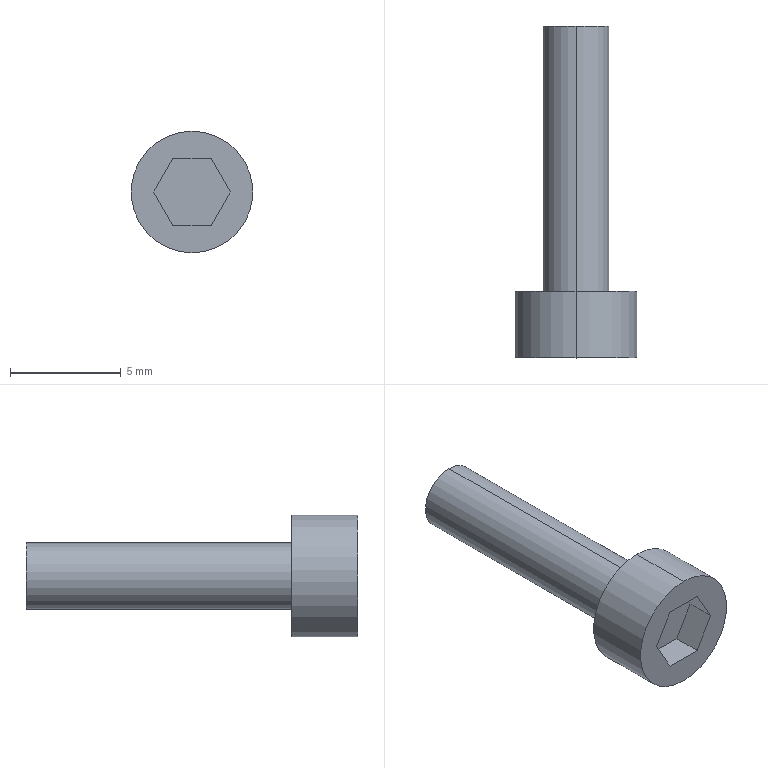Part | SolidWorks | features BaseBody 1 | 1 solid | 14 faces | box 5.5 x 15 x 5.5 mm | volume 145.965 mm3 | plane 10 | cylinder 4 | commonest cylinder face diameters 3 x2 5.5 x2
STEP:
#1=CARTESIAN_POINT('',(0.,15.,-1.5));
#2=VERTEX_POINT('',#1);
#3=CARTESIAN_POINT('',(0.,15.,1.5));
#4=VERTEX_POINT('',#3);
#5=CARTESIAN_POINT('',(0.,15.,0.));
#6=DIRECTION('',(0.,-1.,0.));
#7=DIRECTION('',(0.,0.,-1.));
#8=AXIS2_PLACEMENT_3D('',#5,#6,#7);
#9=CIRCLE('',#8,1.5);
#10=EDGE_CURVE('',#2,#4,#9,.T.);
#11=ORIENTED_EDGE('',*,*,#10,.T.);
#12=CARTESIAN_POINT('',(0.,3.,1.5));
#13=VERTEX_POINT('',#12);
#14=CARTESIAN_POINT('',(0.,15.,1.5));
#15=DIRECTION('',(0.,-1.,0.));
#16=VECTOR('',#15,1000.);
#17=LINE('',#14,#16);
#18=EDGE_CURVE('',#4,#13,#17,.T.);
#19=ORIENTED_EDGE('',*,*,#18,.T.);
#20=CARTESIAN_POINT('',(0.,3.,-1.5));
#21=VERTEX_POINT('',#20);
#22=CARTESIAN_POINT('',(0.,3.,0.));
#23=DIRECTION('',(0.,1.,0.));
#24=DIRECTION('',(0.,0.,-1.));
#25=AXIS2_PLACEMENT_3D('',#22,#23,#24);
#26=CIRCLE('',#25,1.5);
#27=EDGE_CURVE('',#13,#21,#26,.T.);
#28=ORIENTED_EDGE('',*,*,#27,.T.);
#29=CARTESIAN_POINT('',(0.,15.,-1.5));
#30=DIRECTION('',(0.,-1.,0.));
#31=VECTOR('',#30,1000.);
#32=LINE('',#29,#31);
#33=EDGE_CURVE('',#2,#21,#32,.T.);
#34=ORIENTED_EDGE('',*,*,#33,.F.);
#35=EDGE_LOOP('',(#11,#19,#28,#34));
#36=FACE_OUTER_BOUND('',#35,.T.);
#37=CARTESIAN_POINT('',(0.,15.,0.));
#38=DIRECTION('',(0.,-1.,0.));
#39=DIRECTION('',(0.,0.,-1.));
#40=AXIS2_PLACEMENT_3D('',#37,#38,#39);
#41=CYLINDRICAL_SURFACE('',#40,1.5);
#42=ADVANCED_FACE('',(#36),#41,.T.);
#43=CARTESIAN_POINT('',(0.,3.,2.75));
#44=VERTEX_POINT('',#43);
#45=CARTESIAN_POINT('',(0.,3.,-2.75));
#46=VERTEX_POINT('',#45);
#47=CARTESIAN_POINT('',(0.,3.,0.));
#48=DIRECTION('',(0.,1.,0.));
#49=DIRECTION('',(0.,0.,-1.));
#50=AXIS2_PLACEMENT_3D('',#47,#48,#49);
#51=CIRCLE('',#50,2.75);
#52=EDGE_CURVE('',#44,#46,#51,.T.);
#53=ORIENTED_EDGE('',*,*,#52,.F.);
#54=CARTESIAN_POINT('',(0.,0.,2.75));
#55=VERTEX_POINT('',#54);
#56=CARTESIAN_POINT('',(0.,3.,2.75));
#57=DIRECTION('',(0.,-1.,0.));
#58=VECTOR('',#57,1000.);
#59=LINE('',#56,#58);
#60=EDGE_CURVE('',#44,#55,#59,.T.);
#61=ORIENTED_EDGE('',*,*,#60,.T.);
#62=CARTESIAN_POINT('',(0.,0.,-2.75));
#63=VERTEX_POINT('',#62);
#64=CARTESIAN_POINT('',(0.,0.,0.));
#65=DIRECTION('',(0.,1.,0.));
#66=DIRECTION('',(0.,0.,-1.));
#67=AXIS2_PLACEMENT_3D('',#64,#65,#66);
#68=CIRCLE('',#67,2.75);
#69=EDGE_CURVE('',#55,#63,#68,.T.);
#70=ORIENTED_EDGE('',*,*,#69,.T.);
#71=CARTESIAN_POINT('',(0.,3.,-2.75));
#72=DIRECTION('',(0.,-1.,0.));
#73=VECTOR('',#72,1000.);
#74=LINE('',#71,#73);
#75=EDGE_CURVE('',#46,#63,#74,.T.);
#76=ORIENTED_EDGE('',*,*,#75,.F.);
#77=EDGE_LOOP('',(#53,#61,#70,#76));
#78=FACE_OUTER_BOUND('',#77,.T.);
#79=CARTESIAN_POINT('',(0.,3.,0.));
#80=DIRECTION('',(0.,-1.,0.));
#81=DIRECTION('',(0.,0.,-1.));
#82=AXIS2_PLACEMENT_3D('',#79,#80,#81);
#83=CYLINDRICAL_SURFACE('',#82,2.75);
#84=ADVANCED_FACE('',(#78),#83,.T.);
#85=ORIENTED_EDGE('',*,*,#18,.F.);
#86=CARTESIAN_POINT('',(0.,15.,0.));
#87=DIRECTION('',(0.,-1.,0.));
#88=DIRECTION('',(0.,0.,-1.));
#89=AXIS2_PLACEMENT_3D('',#86,#87,#88);
#90=CIRCLE('',#89,1.5);
#91=EDGE_CURVE('',#4,#2,#90,.T.);
#92=ORIENTED_EDGE('',*,*,#91,.T.);
#93=ORIENTED_EDGE('',*,*,#33,.T.);
#94=CARTESIAN_POINT('',(0.,3.,0.));
#95=DIRECTION('',(0.,1.,0.));
#96=DIRECTION('',(0.,0.,-1.));
#97=AXIS2_PLACEMENT_3D('',#94,#95,#96);
#98=CIRCLE('',#97,1.5);
#99=EDGE_CURVE('',#21,#13,#98,.T.);
#100=ORIENTED_EDGE('',*,*,#99,.T.);
#101=EDGE_LOOP('',(#85,#92,#93,#100));
#102=FACE_OUTER_BOUND('',#101,.T.);
#103=CARTESIAN_POINT('',(0.,15.,0.));
#104=DIRECTION('',(0.,-1.,0.));
#105=DIRECTION('',(0.,0.,-1.));
#106=AXIS2_PLACEMENT_3D('',#103,#104,#105);
#107=CYLINDRICAL_SURFACE('',#106,1.5);
#108=ADVANCED_FACE('',(#102),#107,.T.);
#109=CARTESIAN_POINT('',(0.,3.,0.));
#110=DIRECTION('',(0.,1.,0.));
#111=DIRECTION('',(0.,0.,-1.));
#112=AXIS2_PLACEMENT_3D('',#109,#110,#111);
#113=CIRCLE('',#112,2.75);
#114=EDGE_CURVE('',#46,#44,#113,.T.);
#115=ORIENTED_EDGE('',*,*,#114,.T.);
#116=ORIENTED_EDGE('',*,*,#52,.T.);
#117=EDGE_LOOP('',(#115,#116));
#118=FACE_OUTER_BOUND('',#117,.T.);
#119=ORIENTED_EDGE('',*,*,#99,.F.);
#120=ORIENTED_EDGE('',*,*,#27,.F.);
#121=EDGE_LOOP('',(#119,#120));
#122=FACE_BOUND('',#121,.T.);
#123=CARTESIAN_POINT('',(0.,3.,0.));
#124=DIRECTION('',(0.,1.,0.));
#125=DIRECTION('',(0.,0.,1.));
#126=AXIS2_PLACEMENT_3D('',#123,#124,#125);
#127=PLANE('',#126);
#128=ADVANCED_FACE('',(#118,#122),#127,.T.);
#129=ORIENTED_EDGE('',*,*,#10,.F.);
#130=ORIENTED_EDGE('',*,*,#91,.F.);
#131=EDGE_LOOP('',(#129,#130));
#132=FACE_OUTER_BOUND('',#131,.T.);
#133=CARTESIAN_POINT('',(0.,15.,0.));
#134=DIRECTION('',(0.,1.,0.));
#135=DIRECTION('',(0.,0.,1.));
#136=AXIS2_PLACEMENT_3D('',#133,#134,#135);
#137=PLANE('',#136);
#138=ADVANCED_FACE('',(#132),#137,.T.);
#139=ORIENTED_EDGE('',*,*,#60,.F.);
#140=ORIENTED_EDGE('',*,*,#114,.F.);
#141=ORIENTED_EDGE('',*,*,#75,.T.);
#142=CARTESIAN_POINT('',(0.,0.,0.));
#143=DIRECTION('',(0.,1.,0.));
#144=DIRECTION('',(0.,0.,-1.));
#145=AXIS2_PLACEMENT_3D('',#142,#143,#144);
#146=CIRCLE('',#145,2.75);
#147=EDGE_CURVE('',#63,#55,#146,.T.);
#148=ORIENTED_EDGE('',*,*,#147,.T.);
#149=EDGE_LOOP('',(#139,#140,#141,#148));
#150=FACE_OUTER_BOUND('',#149,.T.);
#151=CARTESIAN_POINT('',(0.,3.,0.));
#152=DIRECTION('',(0.,-1.,0.));
#153=DIRECTION('',(0.,0.,-1.));
#154=AXIS2_PLACEMENT_3D('',#151,#152,#153);
#155=CYLINDRICAL_SURFACE('',#154,2.75);
#156=ADVANCED_FACE('',(#150),#155,.T.);
#157=ORIENTED_EDGE('',*,*,#147,.F.);
#158=ORIENTED_EDGE('',*,*,#69,.F.);
#159=EDGE_LOOP('',(#157,#158));
#160=FACE_OUTER_BOUND('',#159,.T.);
#161=CARTESIAN_POINT('',(0.866,0.,-1.5));
#162=VERTEX_POINT('',#161);
#163=CARTESIAN_POINT('',(1.732,0.,0.));
#164=VERTEX_POINT('',#163);
#165=CARTESIAN_POINT('',(0.866,0.,-1.5));
#166=DIRECTION('',(0.5,0.,0.866));
#167=VECTOR('',#166,1000.);
#168=LINE('',#165,#167);
#169=EDGE_CURVE('',#162,#164,#168,.T.);
#170=ORIENTED_EDGE('',*,*,#169,.F.);
#171=CARTESIAN_POINT('',(-0.866,0.,-1.5));
#172=VERTEX_POINT('',#171);
#173=CARTESIAN_POINT('',(0.,0.,-1.5));
#174=DIRECTION('',(1.,0.,0.));
#175=VECTOR('',#174,1000.);
#176=LINE('',#173,#175);
#177=EDGE_CURVE('',#172,#162,#176,.T.);
#178=ORIENTED_EDGE('',*,*,#177,.F.);
#179=CARTESIAN_POINT('',(-1.732,0.,0.));
#180=VERTEX_POINT('',#179);
#181=CARTESIAN_POINT('',(-1.732,0.,0.));
#182=DIRECTION('',(0.5,0.,-0.866));
#183=VECTOR('',#182,1000.);
#184=LINE('',#181,#183);
#185=EDGE_CURVE('',#180,#172,#184,.T.);
#186=ORIENTED_EDGE('',*,*,#185,.F.);
#187=CARTESIAN_POINT('',(-0.866,0.,1.5));
#188=VERTEX_POINT('',#187);
#189=CARTESIAN_POINT('',(-0.866,0.,1.5));
#190=DIRECTION('',(-0.5,0.,-0.866));
#191=VECTOR('',#190,1000.);
#192=LINE('',#189,#191);
#193=EDGE_CURVE('',#188,#180,#192,.T.);
#194=ORIENTED_EDGE('',*,*,#193,.F.);
#195=CARTESIAN_POINT('',(0.866,0.,1.5));
#196=VERTEX_POINT('',#195);
#197=CARTESIAN_POINT('',(0.,0.,1.5));
#198=DIRECTION('',(-1.,0.,0.));
#199=VECTOR('',#198,1000.);
#200=LINE('',#197,#199);
#201=EDGE_CURVE('',#196,#188,#200,.T.);
#202=ORIENTED_EDGE('',*,*,#201,.F.);
#203=CARTESIAN_POINT('',(1.732,0.,0.));
#204=DIRECTION('',(-0.5,0.,0.866));
#205=VECTOR('',#204,1000.);
#206=LINE('',#203,#205);
#207=EDGE_CURVE('',#164,#196,#206,.T.);
#208=ORIENTED_EDGE('',*,*,#207,.F.);
#209=EDGE_LOOP('',(#170,#178,#186,#194,#202,#208));
#210=FACE_BOUND('',#209,.T.);
#211=CARTESIAN_POINT('',(0.,0.,0.));
#212=DIRECTION('',(0.,1.,0.));
#213=DIRECTION('',(0.,0.,1.));
#214=AXIS2_PLACEMENT_3D('',#211,#212,#213);
#215=PLANE('',#214);
#216=ADVANCED_FACE('',(#160,#210),#215,.F.);
#217=CARTESIAN_POINT('',(0.866,1.3,1.5));
#218=VERTEX_POINT('',#217);
#219=CARTESIAN_POINT('',(0.866,1.3,1.5));
#220=DIRECTION('',(0.,-1.,0.));
#221=VECTOR('',#220,1000.);
#222=LINE('',#219,#221);
#223=EDGE_CURVE('',#218,#196,#222,.T.);
#224=ORIENTED_EDGE('',*,*,#223,.F.);
#225=CARTESIAN_POINT('',(1.732,1.3,0.));
#226=VERTEX_POINT('',#225);
#227=CARTESIAN_POINT('',(1.732,1.3,0.));
#228=DIRECTION('',(-0.5,0.,0.866));
#229=VECTOR('',#228,1000.);
#230=LINE('',#227,#229);
#231=EDGE_CURVE('',#226,#218,#230,.T.);
#232=ORIENTED_EDGE('',*,*,#231,.F.);
#233=CARTESIAN_POINT('',(1.732,1.3,0.));
#234=DIRECTION('',(0.,1.,0.));
#235=VECTOR('',#234,1000.);
#236=LINE('',#233,#235);
#237=EDGE_CURVE('',#164,#226,#236,.T.);
#238=ORIENTED_EDGE('',*,*,#237,.F.);
#239=ORIENTED_EDGE('',*,*,#207,.T.);
#240=EDGE_LOOP('',(#224,#232,#238,#239));
#241=FACE_OUTER_BOUND('',#240,.T.);
#242=CARTESIAN_POINT('',(1.732,1.3,0.));
#243=DIRECTION('',(0.866,0.,0.5));
#244=DIRECTION('',(0.5,0.,-0.866));
#245=AXIS2_PLACEMENT_3D('',#242,#243,#244);
#246=PLANE('',#245);
#247=ADVANCED_FACE('',(#241),#246,.F.);
#248=ORIENTED_EDGE('',*,*,#237,.T.);
#249=CARTESIAN_POINT('',(0.866,1.3,-1.5));
#250=VERTEX_POINT('',#249);
#251=CARTESIAN_POINT('',(0.866,1.3,-1.5));
#252=DIRECTION('',(0.5,0.,0.866));
#253=VECTOR('',#252,1000.);
#254=LINE('',#251,#253);
#255=EDGE_CURVE('',#250,#226,#254,.T.);
#256=ORIENTED_EDGE('',*,*,#255,.F.);
#257=CARTESIAN_POINT('',(0.866,1.3,-1.5));
#258=DIRECTION('',(0.,1.,0.));
#259=VECTOR('',#258,1000.);
#260=LINE('',#257,#259);
#261=EDGE_CURVE('',#162,#250,#260,.T.);
#262=ORIENTED_EDGE('',*,*,#261,.F.);
#263=ORIENTED_EDGE('',*,*,#169,.T.);
#264=EDGE_LOOP('',(#248,#256,#262,#263));
#265=FACE_OUTER_BOUND('',#264,.T.);
#266=CARTESIAN_POINT('',(0.866,1.3,-1.5));
#267=DIRECTION('',(0.866,0.,-0.5));
#268=DIRECTION('',(-0.5,0.,-0.866));
#269=AXIS2_PLACEMENT_3D('',#266,#267,#268);
#270=PLANE('',#269);
#271=ADVANCED_FACE('',(#265),#270,.F.);
#272=ORIENTED_EDGE('',*,*,#261,.T.);
#273=CARTESIAN_POINT('',(-0.866,1.3,-1.5));
#274=VERTEX_POINT('',#273);
#275=CARTESIAN_POINT('',(-0.866,1.3,-1.5));
#276=DIRECTION('',(1.,0.,0.));
#277=VECTOR('',#276,1000.);
#278=LINE('',#275,#277);
#279=EDGE_CURVE('',#274,#250,#278,.T.);
#280=ORIENTED_EDGE('',*,*,#279,.F.);
#281=CARTESIAN_POINT('',(-0.866,1.3,-1.5));
#282=DIRECTION('',(0.,1.,0.));
#283=VECTOR('',#282,1000.);
#284=LINE('',#281,#283);
#285=EDGE_CURVE('',#172,#274,#284,.T.);
#286=ORIENTED_EDGE('',*,*,#285,.F.);
#287=ORIENTED_EDGE('',*,*,#177,.T.);
#288=EDGE_LOOP('',(#272,#280,#286,#287));
#289=FACE_OUTER_BOUND('',#288,.T.);
#290=CARTESIAN_POINT('',(-0.866,1.3,-1.5));
#291=DIRECTION('',(0.,0.,-1.));
#292=DIRECTION('',(-1.,0.,0.));
#293=AXIS2_PLACEMENT_3D('',#290,#291,#292);
#294=PLANE('',#293);
#295=ADVANCED_FACE('',(#289),#294,.F.);
#296=ORIENTED_EDGE('',*,*,#285,.T.);
#297=CARTESIAN_POINT('',(-1.732,1.3,0.));
#298=VERTEX_POINT('',#297);
#299=CARTESIAN_POINT('',(-1.732,1.3,0.));
#300=DIRECTION('',(0.5,0.,-0.866));
#301=VECTOR('',#300,1000.);
#302=LINE('',#299,#301);
#303=EDGE_CURVE('',#298,#274,#302,.T.);
#304=ORIENTED_EDGE('',*,*,#303,.F.);
#305=CARTESIAN_POINT('',(-1.732,1.3,0.));
#306=DIRECTION('',(0.,1.,0.));
#307=VECTOR('',#306,1000.);
#308=LINE('',#305,#307);
#309=EDGE_CURVE('',#180,#298,#308,.T.);
#310=ORIENTED_EDGE('',*,*,#309,.F.);
#311=ORIENTED_EDGE('',*,*,#185,.T.);
#312=EDGE_LOOP('',(#296,#304,#310,#311));
#313=FACE_OUTER_BOUND('',#312,.T.);
#314=CARTESIAN_POINT('',(-1.732,1.3,0.));
#315=DIRECTION('',(-0.866,0.,-0.5));
#316=DIRECTION('',(-0.5,0.,0.866));
#317=AXIS2_PLACEMENT_3D('',#314,#315,#316);
#318=PLANE('',#317);
#319=ADVANCED_FACE('',(#313),#318,.F.);
#320=ORIENTED_EDGE('',*,*,#309,.T.);
#321=CARTESIAN_POINT('',(-0.866,1.3,1.5));
#322=VERTEX_POINT('',#321);
#323=CARTESIAN_POINT('',(-0.866,1.3,1.5));
#324=DIRECTION('',(-0.5,0.,-0.866));
#325=VECTOR('',#324,1000.);
#326=LINE('',#323,#325);
#327=EDGE_CURVE('',#322,#298,#326,.T.);
#328=ORIENTED_EDGE('',*,*,#327,.F.);
#329=CARTESIAN_POINT('',(-0.866,1.3,1.5));
#330=DIRECTION('',(0.,1.,0.));
#331=VECTOR('',#330,1000.);
#332=LINE('',#329,#331);
#333=EDGE_CURVE('',#188,#322,#332,.T.);
#334=ORIENTED_EDGE('',*,*,#333,.F.);
#335=ORIENTED_EDGE('',*,*,#193,.T.);
#336=EDGE_LOOP('',(#320,#328,#334,#335));
#337=FACE_OUTER_BOUND('',#336,.T.);
#338=CARTESIAN_POINT('',(-0.866,1.3,1.5));
#339=DIRECTION('',(-0.866,0.,0.5));
#340=DIRECTION('',(0.5,0.,0.866));
#341=AXIS2_PLACEMENT_3D('',#338,#339,#340);
#342=PLANE('',#341);
#343=ADVANCED_FACE('',(#337),#342,.F.);
#344=ORIENTED_EDGE('',*,*,#333,.T.);
#345=CARTESIAN_POINT('',(0.866,1.3,1.5));
#346=DIRECTION('',(-1.,0.,0.));
#347=VECTOR('',#346,1000.);
#348=LINE('',#345,#347);
#349=EDGE_CURVE('',#218,#322,#348,.T.);
#350=ORIENTED_EDGE('',*,*,#349,.F.);
#351=ORIENTED_EDGE('',*,*,#223,.T.);
#352=ORIENTED_EDGE('',*,*,#201,.T.);
#353=EDGE_LOOP('',(#344,#350,#351,#352));
#354=FACE_OUTER_BOUND('',#353,.T.);
#355=CARTESIAN_POINT('',(0.866,1.3,1.5));
#356=DIRECTION('',(0.,0.,1.));
#357=DIRECTION('',(1.,0.,0.));
#358=AXIS2_PLACEMENT_3D('',#355,#356,#357);
#359=PLANE('',#358);
#360=ADVANCED_FACE('',(#354),#359,.F.);
#361=ORIENTED_EDGE('',*,*,#303,.T.);
#362=ORIENTED_EDGE('',*,*,#279,.T.);
#363=ORIENTED_EDGE('',*,*,#255,.T.);
#364=ORIENTED_EDGE('',*,*,#231,.T.);
#365=ORIENTED_EDGE('',*,*,#349,.T.);
#366=ORIENTED_EDGE('',*,*,#327,.T.);
#367=EDGE_LOOP('',(#361,#362,#363,#364,#365,#366));
#368=FACE_OUTER_BOUND('',#367,.T.);
#369=CARTESIAN_POINT('',(0.,1.3,0.));
#370=DIRECTION('',(0.,-1.,0.));
#371=DIRECTION('',(0.,0.,-1.));
#372=AXIS2_PLACEMENT_3D('',#369,#370,#371);
#373=PLANE('',#372);
#374=ADVANCED_FACE('',(#368),#373,.T.);
#375=CLOSED_SHELL('',(#42,#84,#108,#128,#138,#156,#216,#247,#271,#295,#319,#343,#360,#374));
#376=MANIFOLD_SOLID_BREP('',#375);
#377=CARTESIAN_POINT('',(0.,0.,0.));
#378=DIRECTION('',(0.,0.,1.));
#379=DIRECTION('',(1.,0.,0.));
#380=AXIS2_PLACEMENT_3D('',#377,#378,#379);
#381=(LENGTH_UNIT()NAMED_UNIT(*)SI_UNIT(.MILLI.,.METRE.));
#382=UNCERTAINTY_MEASURE_WITH_UNIT(LENGTH_MEASURE(0.00001),#381,'','');
#383=(NAMED_UNIT(*)PLANE_ANGLE_UNIT()SI_UNIT($,.RADIAN.));
#384=(NAMED_UNIT(*)SI_UNIT($,.STERADIAN.)SOLID_ANGLE_UNIT());
#385=(GEOMETRIC_REPRESENTATION_CONTEXT(3)GLOBAL_UNCERTAINTY_ASSIGNED_CONTEXT((#382))GLOBAL_UNIT_ASSIGNED_CONTEXT((#381,#383,#384))REPRESENTATION_CONTEXT('',''));
#386=ADVANCED_BREP_SHAPE_REPRESENTATION('',(#376,#380),#385);